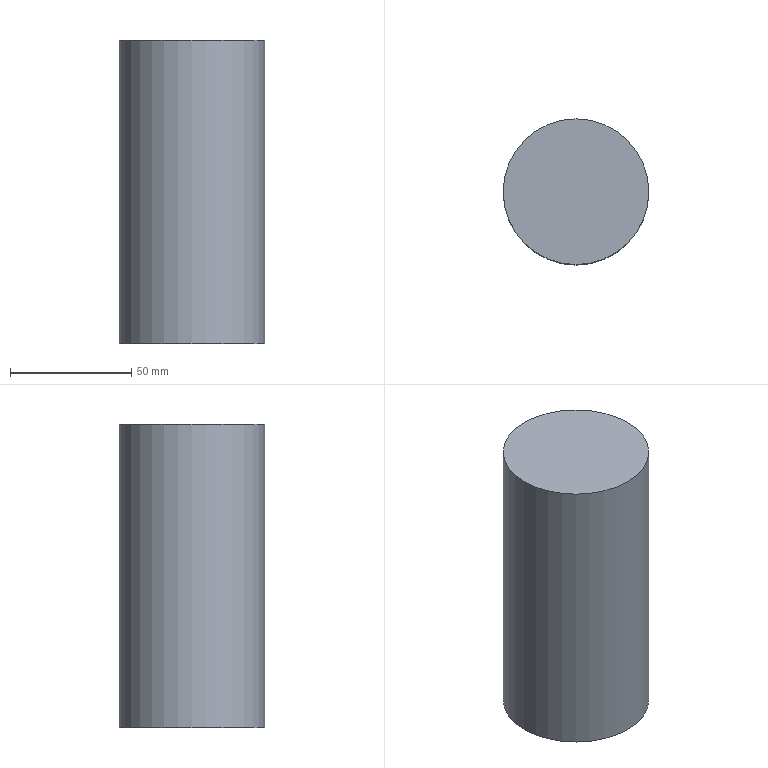Part | NX | features solid 2 | 1 solid | 3 faces | box 60 x 60 x 125 mm | volume 353429 mm3 | plane 2 | cylinder 1 | commonest cylinder face diameters 60 x1
STEP:
#1=CARTESIAN_POINT('',(-140.,-190.,195.));
#2=VERTEX_POINT('',#1);
#3=CARTESIAN_POINT('',(-170.,-190.,195.));
#4=DIRECTION('',(0.,0.,1.));
#5=DIRECTION('',(1.,0.,0.));
#6=AXIS2_PLACEMENT_3D('',#3,#4,#5);
#7=CIRCLE('',#6,30.);
#8=EDGE_CURVE('',#2,#2,#7,.T.);
#9=ORIENTED_EDGE('',*,*,#8,.T.);
#10=EDGE_LOOP('',(#9));
#11=FACE_BOUND('',#10,.T.);
#12=CARTESIAN_POINT('',(-140.,-190.,320.));
#13=VERTEX_POINT('',#12);
#14=CARTESIAN_POINT('',(-170.,-190.,320.));
#15=DIRECTION('',(0.,0.,1.));
#16=DIRECTION('',(1.,0.,0.));
#17=AXIS2_PLACEMENT_3D('',#14,#15,#16);
#18=CIRCLE('',#17,30.);
#19=EDGE_CURVE('',#13,#13,#18,.T.);
#20=ORIENTED_EDGE('',*,*,#19,.F.);
#21=EDGE_LOOP('',(#20));
#22=FACE_BOUND('',#21,.T.);
#23=CARTESIAN_POINT('',(-170.,-190.,155.));
#24=DIRECTION('',(0.,0.,1.));
#25=DIRECTION('',(1.,0.,0.));
#26=AXIS2_PLACEMENT_3D('',#23,#24,#25);
#27=CYLINDRICAL_SURFACE('',#26,30.);
#28=ADVANCED_FACE('',(#11,#22),#27,.T.);
#29=ORIENTED_EDGE('',*,*,#8,.F.);
#30=EDGE_LOOP('',(#29));
#31=FACE_BOUND('',#30,.T.);
#32=CARTESIAN_POINT('',(-170.,-190.,195.));
#33=DIRECTION('',(0.,0.,1.));
#34=DIRECTION('',(1.,0.,0.));
#35=AXIS2_PLACEMENT_3D('',#32,#33,#34);
#36=PLANE('',#35);
#37=ADVANCED_FACE('',(#31),#36,.F.);
#38=ORIENTED_EDGE('',*,*,#19,.T.);
#39=EDGE_LOOP('',(#38));
#40=FACE_BOUND('',#39,.T.);
#41=CARTESIAN_POINT('',(-170.,-190.,320.));
#42=DIRECTION('',(0.,0.,1.));
#43=DIRECTION('',(1.,0.,0.));
#44=AXIS2_PLACEMENT_3D('',#41,#42,#43);
#45=PLANE('',#44);
#46=ADVANCED_FACE('',(#40),#45,.T.);
#47=CLOSED_SHELL('',(#28,#37,#46));
#48=MANIFOLD_SOLID_BREP('',#47);
#49=(LENGTH_UNIT()NAMED_UNIT(*)SI_UNIT(.MILLI.,.METRE.));
#50=UNCERTAINTY_MEASURE_WITH_UNIT(LENGTH_MEASURE(0.00001),#49,'','');
#51=(NAMED_UNIT(*)PLANE_ANGLE_UNIT()SI_UNIT($,.RADIAN.));
#52=(NAMED_UNIT(*)SI_UNIT($,.STERADIAN.)SOLID_ANGLE_UNIT());
#53=(GEOMETRIC_REPRESENTATION_CONTEXT(3)GLOBAL_UNCERTAINTY_ASSIGNED_CONTEXT((#50))GLOBAL_UNIT_ASSIGNED_CONTEXT((#49,#51,#52))REPRESENTATION_CONTEXT('',''));
#54=ADVANCED_BREP_SHAPE_REPRESENTATION('',(#48),#53);